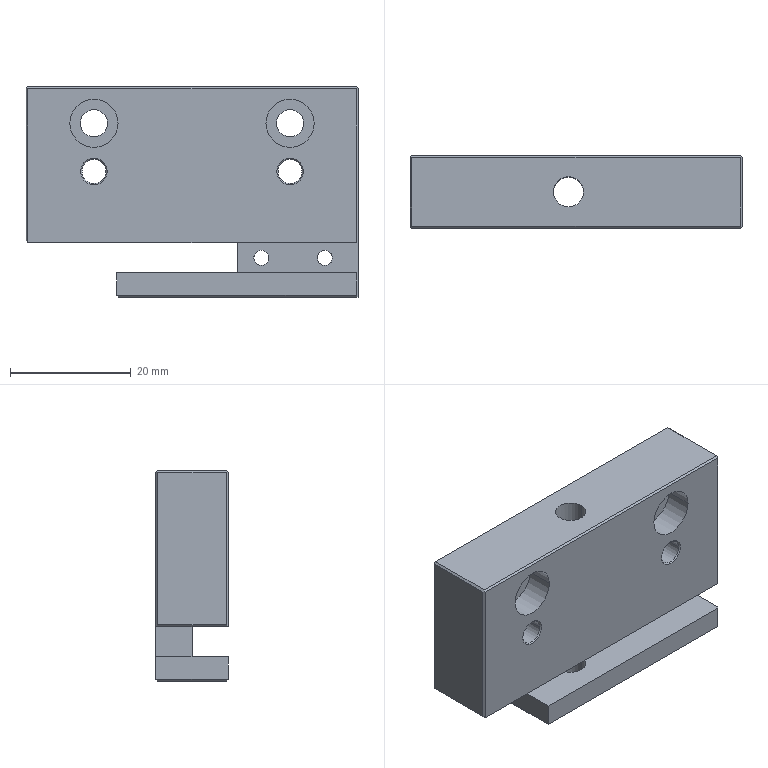Part | NX | 1 solid | 59 faces | box 55 x 12 x 34.8 mm | volume 17876 mm3 | plane 27 | cylinder 22 | cone 10 | commonest cylinder face diameters 2.5 x6 4 x4 4.5 x4 5 x4 8 x4